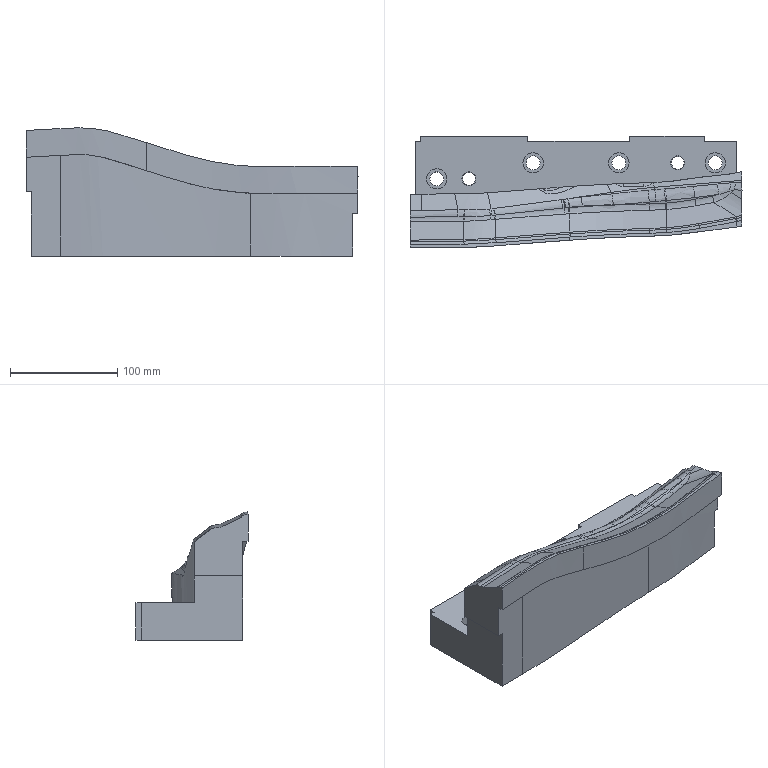Part | NX | features solid 2 | 1 solid | 138 faces | box 310.036 x 104.591 x 119.835 mm | volume 1667578 mm3 | spline 53 | cylinder 51 | plane 34 | commonest cylinder face diameters 20 x8 13 x6 12 x4 19 x4 20.001 x4 10 x3